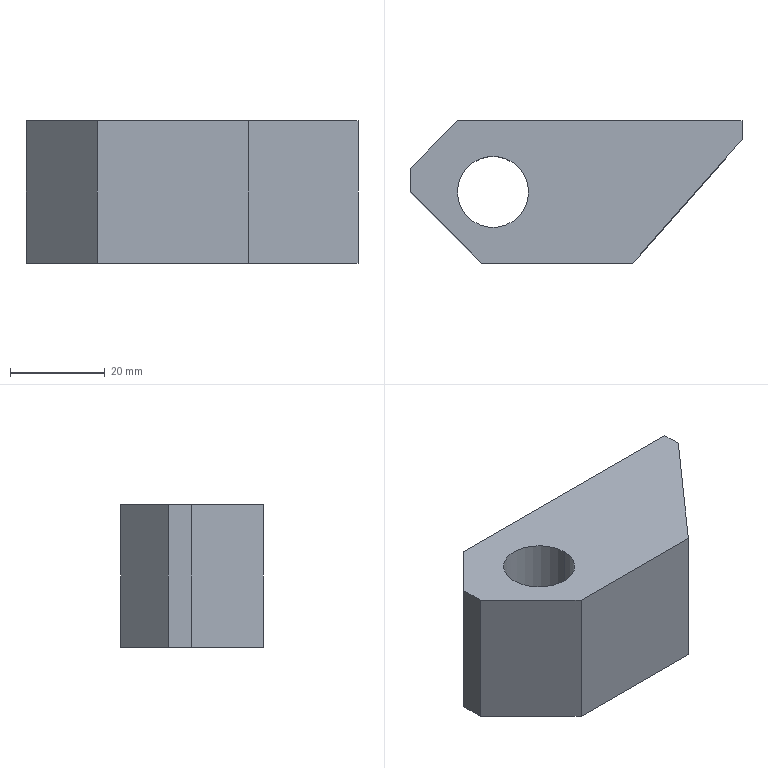Part | SolidWorks | features BaseBody 1 | 1 solid | 11 faces | box 70 x 30 x 30 mm | volume 43854 mm3 | plane 9 | cylinder 2 | commonest cylinder face diameters 15 x2
STEP:
#1=CARTESIAN_POINT('',(-25.,0.,-15.));
#2=VERTEX_POINT('',#1);
#3=CARTESIAN_POINT('',(-10.,0.,-15.));
#4=VERTEX_POINT('',#3);
#5=CARTESIAN_POINT('',(-17.5,0.,-15.));
#6=DIRECTION('',(0.,0.,1.));
#7=DIRECTION('',(1.,0.,0.));
#8=AXIS2_PLACEMENT_3D('',#5,#6,#7);
#9=CIRCLE('',#8,7.5);
#10=EDGE_CURVE('',#2,#4,#9,.T.);
#11=ORIENTED_EDGE('',*,*,#10,.F.);
#12=CARTESIAN_POINT('',(-25.,0.,15.));
#13=VERTEX_POINT('',#12);
#14=CARTESIAN_POINT('',(-25.,0.,-15.));
#15=DIRECTION('',(0.,0.,1.));
#16=VECTOR('',#15,1000.);
#17=LINE('',#14,#16);
#18=EDGE_CURVE('',#2,#13,#17,.T.);
#19=ORIENTED_EDGE('',*,*,#18,.T.);
#20=CARTESIAN_POINT('',(-10.,0.,15.));
#21=VERTEX_POINT('',#20);
#22=CARTESIAN_POINT('',(-17.5,0.,15.));
#23=DIRECTION('',(0.,0.,1.));
#24=DIRECTION('',(1.,0.,0.));
#25=AXIS2_PLACEMENT_3D('',#22,#23,#24);
#26=CIRCLE('',#25,7.5);
#27=EDGE_CURVE('',#13,#21,#26,.T.);
#28=ORIENTED_EDGE('',*,*,#27,.T.);
#29=CARTESIAN_POINT('',(-10.,0.,-15.));
#30=DIRECTION('',(0.,0.,1.));
#31=VECTOR('',#30,1000.);
#32=LINE('',#29,#31);
#33=EDGE_CURVE('',#4,#21,#32,.T.);
#34=ORIENTED_EDGE('',*,*,#33,.F.);
#35=EDGE_LOOP('',(#11,#19,#28,#34));
#36=FACE_OUTER_BOUND('',#35,.T.);
#37=CARTESIAN_POINT('',(-17.5,0.,-15.));
#38=DIRECTION('',(0.,0.,1.));
#39=DIRECTION('',(1.,0.,0.));
#40=AXIS2_PLACEMENT_3D('',#37,#38,#39);
#41=CYLINDRICAL_SURFACE('',#40,7.5);
#42=ADVANCED_FACE('',(#36),#41,.F.);
#43=CARTESIAN_POINT('',(-35.,5.,15.));
#44=VERTEX_POINT('',#43);
#45=CARTESIAN_POINT('',(-35.,0.,15.));
#46=VERTEX_POINT('',#45);
#47=CARTESIAN_POINT('',(-35.,15.,15.));
#48=DIRECTION('',(0.,-1.,0.));
#49=VECTOR('',#48,1000.);
#50=LINE('',#47,#49);
#51=EDGE_CURVE('',#44,#46,#50,.T.);
#52=ORIENTED_EDGE('',*,*,#51,.F.);
#53=CARTESIAN_POINT('',(-35.,5.,-15.));
#54=VERTEX_POINT('',#53);
#55=CARTESIAN_POINT('',(-35.,5.,15.));
#56=DIRECTION('',(0.,0.,-1.));
#57=VECTOR('',#56,1000.);
#58=LINE('',#55,#57);
#59=EDGE_CURVE('',#44,#54,#58,.T.);
#60=ORIENTED_EDGE('',*,*,#59,.T.);
#61=CARTESIAN_POINT('',(-35.,0.,-15.));
#62=VERTEX_POINT('',#61);
#63=CARTESIAN_POINT('',(-35.,15.,-15.));
#64=DIRECTION('',(0.,-1.,0.));
#65=VECTOR('',#64,1000.);
#66=LINE('',#63,#65);
#67=EDGE_CURVE('',#54,#62,#66,.T.);
#68=ORIENTED_EDGE('',*,*,#67,.T.);
#69=CARTESIAN_POINT('',(-35.,0.,15.));
#70=DIRECTION('',(0.,0.,1.));
#71=VECTOR('',#70,1000.);
#72=LINE('',#69,#71);
#73=EDGE_CURVE('',#62,#46,#72,.T.);
#74=ORIENTED_EDGE('',*,*,#73,.T.);
#75=EDGE_LOOP('',(#52,#60,#68,#74));
#76=FACE_OUTER_BOUND('',#75,.T.);
#77=CARTESIAN_POINT('',(-35.,15.,15.));
#78=DIRECTION('',(1.,0.,0.));
#79=DIRECTION('',(0.,0.,-1.));
#80=AXIS2_PLACEMENT_3D('',#77,#78,#79);
#81=PLANE('',#80);
#82=ADVANCED_FACE('',(#76),#81,.F.);
#83=CARTESIAN_POINT('',(-20.,-15.,15.));
#84=VERTEX_POINT('',#83);
#85=CARTESIAN_POINT('',(12.,-15.,15.));
#86=VERTEX_POINT('',#85);
#87=CARTESIAN_POINT('',(35.,-15.,15.));
#88=DIRECTION('',(1.,0.,0.));
#89=VECTOR('',#88,1000.);
#90=LINE('',#87,#89);
#91=EDGE_CURVE('',#84,#86,#90,.T.);
#92=ORIENTED_EDGE('',*,*,#91,.F.);
#93=CARTESIAN_POINT('',(-20.,-15.,-15.));
#94=VERTEX_POINT('',#93);
#95=CARTESIAN_POINT('',(-20.,-15.,15.));
#96=DIRECTION('',(0.,0.,-1.));
#97=VECTOR('',#96,1000.);
#98=LINE('',#95,#97);
#99=EDGE_CURVE('',#84,#94,#98,.T.);
#100=ORIENTED_EDGE('',*,*,#99,.T.);
#101=CARTESIAN_POINT('',(12.,-15.,-15.));
#102=VERTEX_POINT('',#101);
#103=CARTESIAN_POINT('',(35.,-15.,-15.));
#104=DIRECTION('',(1.,0.,0.));
#105=VECTOR('',#104,1000.);
#106=LINE('',#103,#105);
#107=EDGE_CURVE('',#94,#102,#106,.T.);
#108=ORIENTED_EDGE('',*,*,#107,.T.);
#109=CARTESIAN_POINT('',(12.,-15.,-15.));
#110=DIRECTION('',(0.,0.,1.));
#111=VECTOR('',#110,1000.);
#112=LINE('',#109,#111);
#113=EDGE_CURVE('',#102,#86,#112,.T.);
#114=ORIENTED_EDGE('',*,*,#113,.T.);
#115=EDGE_LOOP('',(#92,#100,#108,#114));
#116=FACE_OUTER_BOUND('',#115,.T.);
#117=CARTESIAN_POINT('',(35.,-15.,15.));
#118=DIRECTION('',(0.,1.,0.));
#119=DIRECTION('',(-1.,0.,0.));
#120=AXIS2_PLACEMENT_3D('',#117,#118,#119);
#121=PLANE('',#120);
#122=ADVANCED_FACE('',(#116),#121,.F.);
#123=CARTESIAN_POINT('',(35.,11.,15.));
#124=VERTEX_POINT('',#123);
#125=CARTESIAN_POINT('',(35.,15.,15.));
#126=VERTEX_POINT('',#125);
#127=CARTESIAN_POINT('',(35.,15.,15.));
#128=DIRECTION('',(0.,1.,0.));
#129=VECTOR('',#128,1000.);
#130=LINE('',#127,#129);
#131=EDGE_CURVE('',#124,#126,#130,.T.);
#132=ORIENTED_EDGE('',*,*,#131,.F.);
#133=CARTESIAN_POINT('',(35.,11.,-15.));
#134=VERTEX_POINT('',#133);
#135=CARTESIAN_POINT('',(35.,11.,-15.));
#136=DIRECTION('',(0.,0.,1.));
#137=VECTOR('',#136,1000.);
#138=LINE('',#135,#137);
#139=EDGE_CURVE('',#134,#124,#138,.T.);
#140=ORIENTED_EDGE('',*,*,#139,.F.);
#141=CARTESIAN_POINT('',(35.,15.,-15.));
#142=VERTEX_POINT('',#141);
#143=CARTESIAN_POINT('',(35.,15.,-15.));
#144=DIRECTION('',(0.,1.,0.));
#145=VECTOR('',#144,1000.);
#146=LINE('',#143,#145);
#147=EDGE_CURVE('',#134,#142,#146,.T.);
#148=ORIENTED_EDGE('',*,*,#147,.T.);
#149=CARTESIAN_POINT('',(35.,15.,15.));
#150=DIRECTION('',(0.,0.,-1.));
#151=VECTOR('',#150,1000.);
#152=LINE('',#149,#151);
#153=EDGE_CURVE('',#126,#142,#152,.T.);
#154=ORIENTED_EDGE('',*,*,#153,.F.);
#155=EDGE_LOOP('',(#132,#140,#148,#154));
#156=FACE_OUTER_BOUND('',#155,.T.);
#157=CARTESIAN_POINT('',(35.,15.,15.));
#158=DIRECTION('',(-1.,0.,0.));
#159=DIRECTION('',(0.,0.,1.));
#160=AXIS2_PLACEMENT_3D('',#157,#158,#159);
#161=PLANE('',#160);
#162=ADVANCED_FACE('',(#156),#161,.F.);
#163=CARTESIAN_POINT('',(-25.,15.,-15.));
#164=VERTEX_POINT('',#163);
#165=CARTESIAN_POINT('',(35.,15.,-15.));
#166=DIRECTION('',(-1.,0.,0.));
#167=VECTOR('',#166,1000.);
#168=LINE('',#165,#167);
#169=EDGE_CURVE('',#142,#164,#168,.T.);
#170=ORIENTED_EDGE('',*,*,#169,.T.);
#171=CARTESIAN_POINT('',(-25.,15.,15.));
#172=VERTEX_POINT('',#171);
#173=CARTESIAN_POINT('',(-25.,15.,15.));
#174=DIRECTION('',(0.,0.,1.));
#175=VECTOR('',#174,1000.);
#176=LINE('',#173,#175);
#177=EDGE_CURVE('',#164,#172,#176,.T.);
#178=ORIENTED_EDGE('',*,*,#177,.T.);
#179=CARTESIAN_POINT('',(35.,15.,15.));
#180=DIRECTION('',(-1.,0.,0.));
#181=VECTOR('',#180,1000.);
#182=LINE('',#179,#181);
#183=EDGE_CURVE('',#126,#172,#182,.T.);
#184=ORIENTED_EDGE('',*,*,#183,.F.);
#185=ORIENTED_EDGE('',*,*,#153,.T.);
#186=EDGE_LOOP('',(#170,#178,#184,#185));
#187=FACE_OUTER_BOUND('',#186,.T.);
#188=CARTESIAN_POINT('',(35.,15.,15.));
#189=DIRECTION('',(0.,-1.,0.));
#190=DIRECTION('',(1.,0.,0.));
#191=AXIS2_PLACEMENT_3D('',#188,#189,#190);
#192=PLANE('',#191);
#193=ADVANCED_FACE('',(#187),#192,.F.);
#194=CARTESIAN_POINT('',(-17.5,0.,15.));
#195=DIRECTION('',(0.,0.,1.));
#196=DIRECTION('',(1.,0.,0.));
#197=AXIS2_PLACEMENT_3D('',#194,#195,#196);
#198=CIRCLE('',#197,7.5);
#199=EDGE_CURVE('',#21,#13,#198,.T.);
#200=ORIENTED_EDGE('',*,*,#199,.F.);
#201=ORIENTED_EDGE('',*,*,#27,.F.);
#202=EDGE_LOOP('',(#200,#201));
#203=FACE_BOUND('',#202,.T.);
#204=ORIENTED_EDGE('',*,*,#183,.T.);
#205=CARTESIAN_POINT('',(-35.,5.,15.));
#206=DIRECTION('',(-0.7071,-0.7071,0.));
#207=VECTOR('',#206,1000.);
#208=LINE('',#205,#207);
#209=EDGE_CURVE('',#172,#44,#208,.T.);
#210=ORIENTED_EDGE('',*,*,#209,.T.);
#211=ORIENTED_EDGE('',*,*,#51,.T.);
#212=CARTESIAN_POINT('',(-20.,-15.,15.));
#213=DIRECTION('',(0.7071,-0.7071,0.));
#214=VECTOR('',#213,1000.);
#215=LINE('',#212,#214);
#216=EDGE_CURVE('',#46,#84,#215,.T.);
#217=ORIENTED_EDGE('',*,*,#216,.T.);
#218=ORIENTED_EDGE('',*,*,#91,.T.);
#219=CARTESIAN_POINT('',(35.,11.,15.));
#220=DIRECTION('',(-0.6626,-0.749,0.));
#221=VECTOR('',#220,1000.);
#222=LINE('',#219,#221);
#223=EDGE_CURVE('',#124,#86,#222,.T.);
#224=ORIENTED_EDGE('',*,*,#223,.F.);
#225=ORIENTED_EDGE('',*,*,#131,.T.);
#226=EDGE_LOOP('',(#204,#210,#211,#217,#218,#224,#225));
#227=FACE_OUTER_BOUND('',#226,.T.);
#228=CARTESIAN_POINT('',(-35.,-15.,15.));
#229=DIRECTION('',(0.,0.,-1.));
#230=DIRECTION('',(-1.,0.,0.));
#231=AXIS2_PLACEMENT_3D('',#228,#229,#230);
#232=PLANE('',#231);
#233=ADVANCED_FACE('',(#203,#227),#232,.F.);
#234=CARTESIAN_POINT('',(-17.5,0.,-15.));
#235=DIRECTION('',(0.,0.,1.));
#236=DIRECTION('',(1.,0.,0.));
#237=AXIS2_PLACEMENT_3D('',#234,#235,#236);
#238=CIRCLE('',#237,7.5);
#239=EDGE_CURVE('',#4,#2,#238,.T.);
#240=ORIENTED_EDGE('',*,*,#239,.T.);
#241=ORIENTED_EDGE('',*,*,#10,.T.);
#242=EDGE_LOOP('',(#240,#241));
#243=FACE_BOUND('',#242,.T.);
#244=ORIENTED_EDGE('',*,*,#67,.F.);
#245=CARTESIAN_POINT('',(-45.,-5.,-15.));
#246=DIRECTION('',(0.7071,0.7071,0.));
#247=VECTOR('',#246,1000.);
#248=LINE('',#245,#247);
#249=EDGE_CURVE('',#54,#164,#248,.T.);
#250=ORIENTED_EDGE('',*,*,#249,.T.);
#251=ORIENTED_EDGE('',*,*,#169,.F.);
#252=ORIENTED_EDGE('',*,*,#147,.F.);
#253=CARTESIAN_POINT('',(35.,11.,-15.));
#254=DIRECTION('',(-0.6626,-0.749,0.));
#255=VECTOR('',#254,1000.);
#256=LINE('',#253,#255);
#257=EDGE_CURVE('',#134,#102,#256,.T.);
#258=ORIENTED_EDGE('',*,*,#257,.T.);
#259=ORIENTED_EDGE('',*,*,#107,.F.);
#260=CARTESIAN_POINT('',(-27.5,-7.5,-15.));
#261=DIRECTION('',(-0.7071,0.7071,0.));
#262=VECTOR('',#261,1000.);
#263=LINE('',#260,#262);
#264=EDGE_CURVE('',#94,#62,#263,.T.);
#265=ORIENTED_EDGE('',*,*,#264,.T.);
#266=EDGE_LOOP('',(#244,#250,#251,#252,#258,#259,#265));
#267=FACE_OUTER_BOUND('',#266,.T.);
#268=CARTESIAN_POINT('',(-35.,-15.,-15.));
#269=DIRECTION('',(0.,0.,-1.));
#270=DIRECTION('',(-1.,0.,0.));
#271=AXIS2_PLACEMENT_3D('',#268,#269,#270);
#272=PLANE('',#271);
#273=ADVANCED_FACE('',(#243,#267),#272,.T.);
#274=ORIENTED_EDGE('',*,*,#223,.T.);
#275=ORIENTED_EDGE('',*,*,#113,.F.);
#276=ORIENTED_EDGE('',*,*,#257,.F.);
#277=ORIENTED_EDGE('',*,*,#139,.T.);
#278=EDGE_LOOP('',(#274,#275,#276,#277));
#279=FACE_OUTER_BOUND('',#278,.T.);
#280=CARTESIAN_POINT('',(35.,11.,-15.));
#281=DIRECTION('',(-0.749,0.6626,0.));
#282=DIRECTION('',(-0.6626,-0.749,0.));
#283=AXIS2_PLACEMENT_3D('',#280,#281,#282);
#284=PLANE('',#283);
#285=ADVANCED_FACE('',(#279),#284,.F.);
#286=ORIENTED_EDGE('',*,*,#18,.F.);
#287=ORIENTED_EDGE('',*,*,#239,.F.);
#288=ORIENTED_EDGE('',*,*,#33,.T.);
#289=ORIENTED_EDGE('',*,*,#199,.T.);
#290=EDGE_LOOP('',(#286,#287,#288,#289));
#291=FACE_OUTER_BOUND('',#290,.T.);
#292=CARTESIAN_POINT('',(-17.5,0.,-15.));
#293=DIRECTION('',(0.,0.,1.));
#294=DIRECTION('',(1.,0.,0.));
#295=AXIS2_PLACEMENT_3D('',#292,#293,#294);
#296=CYLINDRICAL_SURFACE('',#295,7.5);
#297=ADVANCED_FACE('',(#291),#296,.F.);
#298=ORIENTED_EDGE('',*,*,#216,.F.);
#299=ORIENTED_EDGE('',*,*,#73,.F.);
#300=ORIENTED_EDGE('',*,*,#264,.F.);
#301=ORIENTED_EDGE('',*,*,#99,.F.);
#302=EDGE_LOOP('',(#298,#299,#300,#301));
#303=FACE_OUTER_BOUND('',#302,.T.);
#304=CARTESIAN_POINT('',(-20.,-15.,15.));
#305=DIRECTION('',(0.7071,0.7071,0.));
#306=DIRECTION('',(-0.7071,0.7071,0.));
#307=AXIS2_PLACEMENT_3D('',#304,#305,#306);
#308=PLANE('',#307);
#309=ADVANCED_FACE('',(#303),#308,.F.);
#310=ORIENTED_EDGE('',*,*,#209,.F.);
#311=ORIENTED_EDGE('',*,*,#177,.F.);
#312=ORIENTED_EDGE('',*,*,#249,.F.);
#313=ORIENTED_EDGE('',*,*,#59,.F.);
#314=EDGE_LOOP('',(#310,#311,#312,#313));
#315=FACE_OUTER_BOUND('',#314,.T.);
#316=CARTESIAN_POINT('',(-35.,5.,15.));
#317=DIRECTION('',(0.7071,-0.7071,0.));
#318=DIRECTION('',(0.,0.,-1.));
#319=AXIS2_PLACEMENT_3D('',#316,#317,#318);
#320=PLANE('',#319);
#321=ADVANCED_FACE('',(#315),#320,.F.);
#322=CLOSED_SHELL('',(#42,#82,#122,#162,#193,#233,#273,#285,#297,#309,#321));
#323=MANIFOLD_SOLID_BREP('',#322);
#324=CARTESIAN_POINT('',(0.,0.,0.));
#325=DIRECTION('',(0.,0.,1.));
#326=DIRECTION('',(1.,0.,0.));
#327=AXIS2_PLACEMENT_3D('',#324,#325,#326);
#328=(LENGTH_UNIT()NAMED_UNIT(*)SI_UNIT(.MILLI.,.METRE.));
#329=UNCERTAINTY_MEASURE_WITH_UNIT(LENGTH_MEASURE(0.00001),#328,'','');
#330=(NAMED_UNIT(*)PLANE_ANGLE_UNIT()SI_UNIT($,.RADIAN.));
#331=(NAMED_UNIT(*)SI_UNIT($,.STERADIAN.)SOLID_ANGLE_UNIT());
#332=(GEOMETRIC_REPRESENTATION_CONTEXT(3)GLOBAL_UNCERTAINTY_ASSIGNED_CONTEXT((#329))GLOBAL_UNIT_ASSIGNED_CONTEXT((#328,#330,#331))REPRESENTATION_CONTEXT('',''));
#333=ADVANCED_BREP_SHAPE_REPRESENTATION('',(#323,#327),#332);